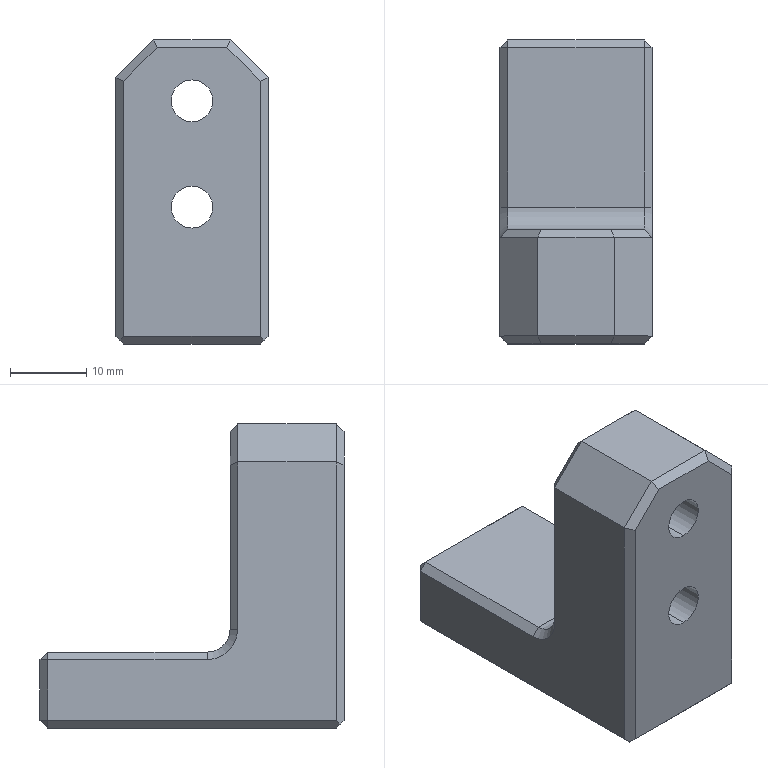Part | Creo | 1 solid | 46 faces | box 20 x 40 x 40 mm | volume 15202 mm3 | plane 35 | cylinder 9 | cone 2 | commonest cylinder face diameters 5.5 x4 9.5 x4 6 x1
STEP:
#1=CARTESIAN_POINT('',(-227.177,374.995,-9.5));
#2=VERTEX_POINT('',#1);
#3=CARTESIAN_POINT('',(-227.177,374.995,24.086));
#4=VERTEX_POINT('',#3);
#5=CARTESIAN_POINT('',(-227.177,374.995,-9.5));
#6=DIRECTION('',(0.,0.,1.));
#7=VECTOR('',#6,33.586);
#8=LINE('',#5,#7);
#9=EDGE_CURVE('',#2,#4,#8,.T.);
#10=ORIENTED_EDGE('',*,*,#9,.T.);
#11=CARTESIAN_POINT('',(-222.763,374.995,28.5));
#12=VERTEX_POINT('',#11);
#13=CARTESIAN_POINT('',(-222.763,374.995,28.5));
#14=DIRECTION('',(-0.7071,0.,-0.7071));
#15=VECTOR('',#14,6.243);
#16=LINE('',#13,#15);
#17=EDGE_CURVE('',#12,#4,#16,.T.);
#18=ORIENTED_EDGE('',*,*,#17,.F.);
#19=CARTESIAN_POINT('',(-213.591,374.995,28.5));
#20=VERTEX_POINT('',#19);
#21=CARTESIAN_POINT('',(-222.763,374.995,28.5));
#22=DIRECTION('',(1.,0.,0.));
#23=VECTOR('',#22,9.172);
#24=LINE('',#21,#23);
#25=EDGE_CURVE('',#12,#20,#24,.T.);
#26=ORIENTED_EDGE('',*,*,#25,.T.);
#27=CARTESIAN_POINT('',(-209.177,374.995,24.086));
#28=VERTEX_POINT('',#27);
#29=CARTESIAN_POINT('',(-209.177,374.995,24.086));
#30=DIRECTION('',(-0.7071,0.,0.7071));
#31=VECTOR('',#30,6.243);
#32=LINE('',#29,#31);
#33=EDGE_CURVE('',#28,#20,#32,.T.);
#34=ORIENTED_EDGE('',*,*,#33,.F.);
#35=CARTESIAN_POINT('',(-209.177,374.995,-9.5));
#36=VERTEX_POINT('',#35);
#37=CARTESIAN_POINT('',(-209.177,374.995,24.086));
#38=DIRECTION('',(0.,0.,-1.));
#39=VECTOR('',#38,33.586);
#40=LINE('',#37,#39);
#41=EDGE_CURVE('',#28,#36,#40,.T.);
#42=ORIENTED_EDGE('',*,*,#41,.T.);
#43=CARTESIAN_POINT('',(-209.177,374.995,-9.5));
#44=DIRECTION('',(-1.,0.,0.));
#45=VECTOR('',#44,18.);
#46=LINE('',#43,#45);
#47=EDGE_CURVE('',#36,#2,#46,.T.);
#48=ORIENTED_EDGE('',*,*,#47,.T.);
#49=EDGE_LOOP('',(#10,#18,#26,#34,#42,#48));
#50=FACE_OUTER_BOUND('',#49,.F.);
#51=CARTESIAN_POINT('',(-218.177,374.995,4.75));
#52=VERTEX_POINT('',#51);
#53=CARTESIAN_POINT('',(-218.177,374.995,10.25));
#54=VERTEX_POINT('',#53);
#55=CARTESIAN_POINT('',(-218.177,374.995,7.5));
#56=DIRECTION('',(0.,1.,0.));
#57=DIRECTION('',(0.,0.,-1.));
#58=AXIS2_PLACEMENT_3D('',#55,#56,#57);
#59=CIRCLE('',#58,2.75);
#60=EDGE_CURVE('',#52,#54,#59,.T.);
#61=ORIENTED_EDGE('',*,*,#60,.F.);
#62=CARTESIAN_POINT('',(-218.177,374.995,7.5));
#63=DIRECTION('',(0.,1.,0.));
#64=DIRECTION('',(0.,0.,1.));
#65=AXIS2_PLACEMENT_3D('',#62,#63,#64);
#66=CIRCLE('',#65,2.75);
#67=EDGE_CURVE('',#54,#52,#66,.T.);
#68=ORIENTED_EDGE('',*,*,#67,.F.);
#69=EDGE_LOOP('',(#61,#68));
#70=FACE_BOUND('',#69,.F.);
#71=CARTESIAN_POINT('',(-218.177,374.995,18.75));
#72=VERTEX_POINT('',#71);
#73=CARTESIAN_POINT('',(-218.177,374.995,24.25));
#74=VERTEX_POINT('',#73);
#75=CARTESIAN_POINT('',(-218.177,374.995,21.5));
#76=DIRECTION('',(0.,1.,0.));
#77=DIRECTION('',(0.,0.,-1.));
#78=AXIS2_PLACEMENT_3D('',#75,#76,#77);
#79=CIRCLE('',#78,2.75);
#80=EDGE_CURVE('',#72,#74,#79,.T.);
#81=ORIENTED_EDGE('',*,*,#80,.F.);
#82=CARTESIAN_POINT('',(-218.177,374.995,21.5));
#83=DIRECTION('',(0.,1.,0.));
#84=DIRECTION('',(0.,0.,1.));
#85=AXIS2_PLACEMENT_3D('',#82,#83,#84);
#86=CIRCLE('',#85,2.75);
#87=EDGE_CURVE('',#74,#72,#86,.T.);
#88=ORIENTED_EDGE('',*,*,#87,.F.);
#89=EDGE_LOOP('',(#81,#88));
#90=FACE_BOUND('',#89,.F.);
#91=CARTESIAN_POINT('',(-218.177,374.995,12.));
#92=DIRECTION('',(0.,-1.,0.));
#93=DIRECTION('',(0.,0.,-1.));
#94=AXIS2_PLACEMENT_3D('',#91,#92,#93);
#95=PLANE('',#94);
#96=ADVANCED_FACE('',(#50,#70,#90),#95,.T.);
#97=ORIENTED_EDGE('',*,*,#60,.T.);
#98=CARTESIAN_POINT('',(-218.177,383.995,10.25));
#99=VERTEX_POINT('',#98);
#100=CARTESIAN_POINT('',(-218.177,374.995,10.25));
#101=DIRECTION('',(0.,1.,0.));
#102=VECTOR('',#101,9.);
#103=LINE('',#100,#102);
#104=EDGE_CURVE('',#54,#99,#103,.T.);
#105=ORIENTED_EDGE('',*,*,#104,.T.);
#106=CARTESIAN_POINT('',(-218.177,383.995,4.75));
#107=VERTEX_POINT('',#106);
#108=CARTESIAN_POINT('',(-218.177,383.995,7.5));
#109=DIRECTION('',(0.,-1.,0.));
#110=DIRECTION('',(0.,0.,1.));
#111=AXIS2_PLACEMENT_3D('',#108,#109,#110);
#112=CIRCLE('',#111,2.75);
#113=EDGE_CURVE('',#99,#107,#112,.T.);
#114=ORIENTED_EDGE('',*,*,#113,.T.);
#115=CARTESIAN_POINT('',(-218.177,374.995,4.75));
#116=DIRECTION('',(0.,1.,0.));
#117=VECTOR('',#116,9.);
#118=LINE('',#115,#117);
#119=EDGE_CURVE('',#52,#107,#118,.T.);
#120=ORIENTED_EDGE('',*,*,#119,.F.);
#121=EDGE_LOOP('',(#97,#105,#114,#120));
#122=FACE_OUTER_BOUND('',#121,.F.);
#123=CARTESIAN_POINT('',(-218.177,389.995,7.5));
#124=DIRECTION('',(0.,1.,0.));
#125=DIRECTION('',(0.,0.,1.));
#126=AXIS2_PLACEMENT_3D('',#123,#124,#125);
#127=CYLINDRICAL_SURFACE('',#126,2.75);
#128=ADVANCED_FACE('',(#122),#127,.F.);
#129=ORIENTED_EDGE('',*,*,#67,.T.);
#130=ORIENTED_EDGE('',*,*,#119,.T.);
#131=CARTESIAN_POINT('',(-218.177,383.995,7.5));
#132=DIRECTION('',(0.,-1.,0.));
#133=DIRECTION('',(0.,0.,-1.));
#134=AXIS2_PLACEMENT_3D('',#131,#132,#133);
#135=CIRCLE('',#134,2.75);
#136=EDGE_CURVE('',#107,#99,#135,.T.);
#137=ORIENTED_EDGE('',*,*,#136,.T.);
#138=ORIENTED_EDGE('',*,*,#104,.F.);
#139=EDGE_LOOP('',(#129,#130,#137,#138));
#140=FACE_OUTER_BOUND('',#139,.F.);
#141=CARTESIAN_POINT('',(-218.177,389.995,7.5));
#142=DIRECTION('',(0.,1.,0.));
#143=DIRECTION('',(0.,0.,1.));
#144=AXIS2_PLACEMENT_3D('',#141,#142,#143);
#145=CYLINDRICAL_SURFACE('',#144,2.75);
#146=ADVANCED_FACE('',(#140),#145,.F.);
#147=CARTESIAN_POINT('',(-218.177,383.995,2.75));
#148=VERTEX_POINT('',#147);
#149=CARTESIAN_POINT('',(-218.177,383.995,12.25));
#150=VERTEX_POINT('',#149);
#151=CARTESIAN_POINT('',(-218.177,383.995,7.5));
#152=DIRECTION('',(0.,1.,0.));
#153=DIRECTION('',(0.,0.,-1.));
#154=AXIS2_PLACEMENT_3D('',#151,#152,#153);
#155=CIRCLE('',#154,4.75);
#156=EDGE_CURVE('',#148,#150,#155,.T.);
#157=ORIENTED_EDGE('',*,*,#156,.F.);
#158=CARTESIAN_POINT('',(-218.177,383.995,7.5));
#159=DIRECTION('',(0.,1.,0.));
#160=DIRECTION('',(0.,0.,1.));
#161=AXIS2_PLACEMENT_3D('',#158,#159,#160);
#162=CIRCLE('',#161,4.75);
#163=EDGE_CURVE('',#150,#148,#162,.T.);
#164=ORIENTED_EDGE('',*,*,#163,.F.);
#165=EDGE_LOOP('',(#157,#164));
#166=FACE_OUTER_BOUND('',#165,.F.);
#167=ORIENTED_EDGE('',*,*,#136,.F.);
#168=ORIENTED_EDGE('',*,*,#113,.F.);
#169=EDGE_LOOP('',(#167,#168));
#170=FACE_BOUND('',#169,.F.);
#171=CARTESIAN_POINT('',(-222.927,383.995,7.5));
#172=DIRECTION('',(0.,-1.,0.));
#173=DIRECTION('',(0.,0.,-1.));
#174=AXIS2_PLACEMENT_3D('',#171,#172,#173);
#175=PLANE('',#174);
#176=ADVANCED_FACE('',(#166,#170),#175,.F.);
#177=ORIENTED_EDGE('',*,*,#156,.T.);
#178=CARTESIAN_POINT('',(-218.177,389.995,12.25));
#179=VERTEX_POINT('',#178);
#180=CARTESIAN_POINT('',(-218.177,383.995,12.25));
#181=DIRECTION('',(0.,1.,0.));
#182=VECTOR('',#181,6.);
#183=LINE('',#180,#182);
#184=EDGE_CURVE('',#150,#179,#183,.T.);
#185=ORIENTED_EDGE('',*,*,#184,.T.);
#186=CARTESIAN_POINT('',(-218.177,389.995,2.75));
#187=VERTEX_POINT('',#186);
#188=CARTESIAN_POINT('',(-218.177,389.995,7.5));
#189=DIRECTION('',(0.,-1.,0.));
#190=DIRECTION('',(0.,0.,1.));
#191=AXIS2_PLACEMENT_3D('',#188,#189,#190);
#192=CIRCLE('',#191,4.75);
#193=EDGE_CURVE('',#179,#187,#192,.T.);
#194=ORIENTED_EDGE('',*,*,#193,.T.);
#195=CARTESIAN_POINT('',(-218.177,383.995,2.75));
#196=DIRECTION('',(0.,1.,0.));
#197=VECTOR('',#196,6.);
#198=LINE('',#195,#197);
#199=EDGE_CURVE('',#148,#187,#198,.T.);
#200=ORIENTED_EDGE('',*,*,#199,.F.);
#201=EDGE_LOOP('',(#177,#185,#194,#200));
#202=FACE_OUTER_BOUND('',#201,.F.);
#203=CARTESIAN_POINT('',(-218.177,389.995,7.5));
#204=DIRECTION('',(0.,1.,0.));
#205=DIRECTION('',(0.,0.,1.));
#206=AXIS2_PLACEMENT_3D('',#203,#204,#205);
#207=CYLINDRICAL_SURFACE('',#206,4.75);
#208=ADVANCED_FACE('',(#202),#207,.F.);
#209=ORIENTED_EDGE('',*,*,#163,.T.);
#210=ORIENTED_EDGE('',*,*,#199,.T.);
#211=CARTESIAN_POINT('',(-218.177,389.995,7.5));
#212=DIRECTION('',(0.,-1.,0.));
#213=DIRECTION('',(0.,0.,-1.));
#214=AXIS2_PLACEMENT_3D('',#211,#212,#213);
#215=CIRCLE('',#214,4.75);
#216=EDGE_CURVE('',#187,#179,#215,.T.);
#217=ORIENTED_EDGE('',*,*,#216,.T.);
#218=ORIENTED_EDGE('',*,*,#184,.F.);
#219=EDGE_LOOP('',(#209,#210,#217,#218));
#220=FACE_OUTER_BOUND('',#219,.F.);
#221=CARTESIAN_POINT('',(-218.177,389.995,7.5));
#222=DIRECTION('',(0.,1.,0.));
#223=DIRECTION('',(0.,0.,1.));
#224=AXIS2_PLACEMENT_3D('',#221,#222,#223);
#225=CYLINDRICAL_SURFACE('',#224,4.75);
#226=ADVANCED_FACE('',(#220),#225,.F.);
#227=CARTESIAN_POINT('',(-213.591,389.995,28.5));
#228=VERTEX_POINT('',#227);
#229=CARTESIAN_POINT('',(-209.177,389.995,24.086));
#230=VERTEX_POINT('',#229);
#231=CARTESIAN_POINT('',(-213.591,389.995,28.5));
#232=DIRECTION('',(0.7071,0.,-0.7071));
#233=VECTOR('',#232,6.243);
#234=LINE('',#231,#233);
#235=EDGE_CURVE('',#228,#230,#234,.T.);
#236=ORIENTED_EDGE('',*,*,#235,.F.);
#237=CARTESIAN_POINT('',(-222.763,389.995,28.5));
#238=VERTEX_POINT('',#237);
#239=CARTESIAN_POINT('',(-213.591,389.995,28.5));
#240=DIRECTION('',(-1.,0.,0.));
#241=VECTOR('',#240,9.172);
#242=LINE('',#239,#241);
#243=EDGE_CURVE('',#228,#238,#242,.T.);
#244=ORIENTED_EDGE('',*,*,#243,.T.);
#245=CARTESIAN_POINT('',(-227.177,389.995,24.086));
#246=VERTEX_POINT('',#245);
#247=CARTESIAN_POINT('',(-227.177,389.995,24.086));
#248=DIRECTION('',(0.7071,0.,0.7071));
#249=VECTOR('',#248,6.243);
#250=LINE('',#247,#249);
#251=EDGE_CURVE('',#246,#238,#250,.T.);
#252=ORIENTED_EDGE('',*,*,#251,.F.);
#253=CARTESIAN_POINT('',(-227.177,389.995,2.5));
#254=VERTEX_POINT('',#253);
#255=CARTESIAN_POINT('',(-227.177,389.995,24.086));
#256=DIRECTION('',(0.,0.,-1.));
#257=VECTOR('',#256,21.586);
#258=LINE('',#255,#257);
#259=EDGE_CURVE('',#246,#254,#258,.T.);
#260=ORIENTED_EDGE('',*,*,#259,.T.);
#261=CARTESIAN_POINT('',(-209.177,389.995,2.5));
#262=VERTEX_POINT('',#261);
#263=CARTESIAN_POINT('',(-227.177,389.995,2.5));
#264=DIRECTION('',(1.,0.,0.));
#265=VECTOR('',#264,18.);
#266=LINE('',#263,#265);
#267=EDGE_CURVE('',#254,#262,#266,.T.);
#268=ORIENTED_EDGE('',*,*,#267,.T.);
#269=CARTESIAN_POINT('',(-209.177,389.995,2.5));
#270=DIRECTION('',(0.,0.,1.));
#271=VECTOR('',#270,21.586);
#272=LINE('',#269,#271);
#273=EDGE_CURVE('',#262,#230,#272,.T.);
#274=ORIENTED_EDGE('',*,*,#273,.T.);
#275=EDGE_LOOP('',(#236,#244,#252,#260,#268,#274));
#276=FACE_OUTER_BOUND('',#275,.F.);
#277=ORIENTED_EDGE('',*,*,#216,.F.);
#278=ORIENTED_EDGE('',*,*,#193,.F.);
#279=EDGE_LOOP('',(#277,#278));
#280=FACE_BOUND('',#279,.F.);
#281=CARTESIAN_POINT('',(-218.177,389.995,16.75));
#282=VERTEX_POINT('',#281);
#283=CARTESIAN_POINT('',(-218.177,389.995,26.25));
#284=VERTEX_POINT('',#283);
#285=CARTESIAN_POINT('',(-218.177,389.995,21.5));
#286=DIRECTION('',(0.,-1.,0.));
#287=DIRECTION('',(0.,0.,-1.));
#288=AXIS2_PLACEMENT_3D('',#285,#286,#287);
#289=CIRCLE('',#288,4.75);
#290=EDGE_CURVE('',#282,#284,#289,.T.);
#291=ORIENTED_EDGE('',*,*,#290,.F.);
#292=CARTESIAN_POINT('',(-218.177,389.995,21.5));
#293=DIRECTION('',(0.,-1.,0.));
#294=DIRECTION('',(0.,0.,1.));
#295=AXIS2_PLACEMENT_3D('',#292,#293,#294);
#296=CIRCLE('',#295,4.75);
#297=EDGE_CURVE('',#284,#282,#296,.T.);
#298=ORIENTED_EDGE('',*,*,#297,.F.);
#299=EDGE_LOOP('',(#291,#298));
#300=FACE_BOUND('',#299,.F.);
#301=CARTESIAN_POINT('',(-218.177,389.995,27.));
#302=DIRECTION('',(0.,-1.,0.));
#303=DIRECTION('',(0.,0.,-1.));
#304=AXIS2_PLACEMENT_3D('',#301,#302,#303);
#305=PLANE('',#304);
#306=ADVANCED_FACE('',(#276,#280,#300),#305,.F.);
#307=CARTESIAN_POINT('',(-213.177,388.995,29.5));
#308=VERTEX_POINT('',#307);
#309=CARTESIAN_POINT('',(-213.177,388.995,29.5));
#310=DIRECTION('',(-0.2811,0.6786,-0.6786));
#311=VECTOR('',#310,1.474);
#312=LINE('',#309,#311);
#313=EDGE_CURVE('',#308,#228,#312,.T.);
#314=ORIENTED_EDGE('',*,*,#313,.T.);
#315=ORIENTED_EDGE('',*,*,#235,.T.);
#316=CARTESIAN_POINT('',(-208.177,388.995,24.5));
#317=VERTEX_POINT('',#316);
#318=CARTESIAN_POINT('',(-208.177,388.995,24.5));
#319=DIRECTION('',(-0.6786,0.6786,-0.2811));
#320=VECTOR('',#319,1.474);
#321=LINE('',#318,#320);
#322=EDGE_CURVE('',#317,#230,#321,.T.);
#323=ORIENTED_EDGE('',*,*,#322,.F.);
#324=CARTESIAN_POINT('',(-213.177,388.995,29.5));
#325=DIRECTION('',(0.7071,0.,-0.7071));
#326=VECTOR('',#325,7.071);
#327=LINE('',#324,#326);
#328=EDGE_CURVE('',#308,#317,#327,.T.);
#329=ORIENTED_EDGE('',*,*,#328,.F.);
#330=EDGE_LOOP('',(#314,#315,#323,#329));
#331=FACE_OUTER_BOUND('',#330,.F.);
#332=CARTESIAN_POINT('',(-212.634,389.995,27.543));
#333=DIRECTION('',(-0.5,-0.7071,-0.5));
#334=DIRECTION('',(-0.7071,0.,0.7071));
#335=AXIS2_PLACEMENT_3D('',#332,#333,#334);
#336=PLANE('',#335);
#337=ADVANCED_FACE('',(#331),#336,.F.);
#338=ORIENTED_EDGE('',*,*,#313,.F.);
#339=CARTESIAN_POINT('',(-223.177,388.995,29.5));
#340=VERTEX_POINT('',#339);
#341=CARTESIAN_POINT('',(-223.177,388.995,29.5));
#342=DIRECTION('',(1.,0.,0.));
#343=VECTOR('',#342,10.);
#344=LINE('',#341,#343);
#345=EDGE_CURVE('',#340,#308,#344,.T.);
#346=ORIENTED_EDGE('',*,*,#345,.F.);
#347=CARTESIAN_POINT('',(-222.763,389.995,28.5));
#348=DIRECTION('',(-0.2811,-0.6786,0.6786));
#349=VECTOR('',#348,1.474);
#350=LINE('',#347,#349);
#351=EDGE_CURVE('',#238,#340,#350,.T.);
#352=ORIENTED_EDGE('',*,*,#351,.F.);
#353=ORIENTED_EDGE('',*,*,#243,.F.);
#354=EDGE_LOOP('',(#338,#346,#352,#353));
#355=FACE_OUTER_BOUND('',#354,.F.);
#356=CARTESIAN_POINT('',(-218.177,389.995,28.5));
#357=DIRECTION('',(0.,0.7071,0.7071));
#358=DIRECTION('',(1.,0.,0.));
#359=AXIS2_PLACEMENT_3D('',#356,#357,#358);
#360=PLANE('',#359);
#361=ADVANCED_FACE('',(#355),#360,.T.);
#362=CARTESIAN_POINT('',(-213.177,375.995,29.5));
#363=VERTEX_POINT('',#362);
#364=CARTESIAN_POINT('',(-213.177,388.995,29.5));
#365=DIRECTION('',(0.,-1.,0.));
#366=VECTOR('',#365,13.);
#367=LINE('',#364,#366);
#368=EDGE_CURVE('',#308,#363,#367,.T.);
#369=ORIENTED_EDGE('',*,*,#368,.T.);
#370=CARTESIAN_POINT('',(-223.177,375.995,29.5));
#371=VERTEX_POINT('',#370);
#372=CARTESIAN_POINT('',(-213.177,375.995,29.5));
#373=DIRECTION('',(-1.,0.,0.));
#374=VECTOR('',#373,10.);
#375=LINE('',#372,#374);
#376=EDGE_CURVE('',#363,#371,#375,.T.);
#377=ORIENTED_EDGE('',*,*,#376,.T.);
#378=CARTESIAN_POINT('',(-223.177,375.995,29.5));
#379=DIRECTION('',(0.,1.,0.));
#380=VECTOR('',#379,13.);
#381=LINE('',#378,#380);
#382=EDGE_CURVE('',#371,#340,#381,.T.);
#383=ORIENTED_EDGE('',*,*,#382,.T.);
#384=ORIENTED_EDGE('',*,*,#345,.T.);
#385=EDGE_LOOP('',(#369,#377,#383,#384));
#386=FACE_OUTER_BOUND('',#385,.F.);
#387=CARTESIAN_POINT('',(-218.177,333.995,29.5));
#388=DIRECTION('',(0.,0.,1.));
#389=DIRECTION('',(0.,-1.,0.));
#390=AXIS2_PLACEMENT_3D('',#387,#388,#389);
#391=PLANE('',#390);
#392=ADVANCED_FACE('',(#386),#391,.T.);
#393=ORIENTED_EDGE('',*,*,#368,.F.);
#394=ORIENTED_EDGE('',*,*,#328,.T.);
#395=CARTESIAN_POINT('',(-208.177,375.995,24.5));
#396=VERTEX_POINT('',#395);
#397=CARTESIAN_POINT('',(-208.177,375.995,24.5));
#398=DIRECTION('',(0.,1.,0.));
#399=VECTOR('',#398,13.);
#400=LINE('',#397,#399);
#401=EDGE_CURVE('',#396,#317,#400,.T.);
#402=ORIENTED_EDGE('',*,*,#401,.F.);
#403=CARTESIAN_POINT('',(-208.177,375.995,24.5));
#404=DIRECTION('',(-0.7071,0.,0.7071));
#405=VECTOR('',#404,7.071);
#406=LINE('',#403,#405);
#407=EDGE_CURVE('',#396,#363,#406,.T.);
#408=ORIENTED_EDGE('',*,*,#407,.T.);
#409=EDGE_LOOP('',(#393,#394,#402,#408));
#410=FACE_OUTER_BOUND('',#409,.F.);
#411=CARTESIAN_POINT('',(-213.177,333.995,29.5));
#412=DIRECTION('',(-0.7071,0.,-0.7071));
#413=DIRECTION('',(0.,-1.,0.));
#414=AXIS2_PLACEMENT_3D('',#411,#412,#413);
#415=PLANE('',#414);
#416=ADVANCED_FACE('',(#410),#415,.F.);
#417=ORIENTED_EDGE('',*,*,#401,.T.);
#418=CARTESIAN_POINT('',(-208.177,388.995,2.5));
#419=VERTEX_POINT('',#418);
#420=CARTESIAN_POINT('',(-208.177,388.995,24.5));
#421=DIRECTION('',(0.,0.,-1.));
#422=VECTOR('',#421,22.);
#423=LINE('',#420,#422);
#424=EDGE_CURVE('',#317,#419,#423,.T.);
#425=ORIENTED_EDGE('',*,*,#424,.T.);
#426=CARTESIAN_POINT('',(-208.177,392.995,-1.5));
#427=VERTEX_POINT('',#426);
#428=CARTESIAN_POINT('',(-208.177,392.995,2.5));
#429=DIRECTION('',(-1.,0.,0.));
#430=DIRECTION('',(0.,0.,-1.));
#431=AXIS2_PLACEMENT_3D('',#428,#429,#430);
#432=CIRCLE('',#431,4.);
#433=EDGE_CURVE('',#427,#419,#432,.T.);
#434=ORIENTED_EDGE('',*,*,#433,.F.);
#435=CARTESIAN_POINT('',(-208.177,413.995,-1.5));
#436=VERTEX_POINT('',#435);
#437=CARTESIAN_POINT('',(-208.177,392.995,-1.5));
#438=DIRECTION('',(0.,1.,0.));
#439=VECTOR('',#438,21.);
#440=LINE('',#437,#439);
#441=EDGE_CURVE('',#427,#436,#440,.T.);
#442=ORIENTED_EDGE('',*,*,#441,.T.);
#443=CARTESIAN_POINT('',(-208.177,413.995,-9.5));
#444=VERTEX_POINT('',#443);
#445=CARTESIAN_POINT('',(-208.177,413.995,-1.5));
#446=DIRECTION('',(0.,0.,-1.));
#447=VECTOR('',#446,8.);
#448=LINE('',#445,#447);
#449=EDGE_CURVE('',#436,#444,#448,.T.);
#450=ORIENTED_EDGE('',*,*,#449,.T.);
#451=CARTESIAN_POINT('',(-208.177,375.995,-9.5));
#452=VERTEX_POINT('',#451);
#453=CARTESIAN_POINT('',(-208.177,413.995,-9.5));
#454=DIRECTION('',(0.,-1.,0.));
#455=VECTOR('',#454,38.);
#456=LINE('',#453,#455);
#457=EDGE_CURVE('',#444,#452,#456,.T.);
#458=ORIENTED_EDGE('',*,*,#457,.T.);
#459=CARTESIAN_POINT('',(-208.177,375.995,-9.5));
#460=DIRECTION('',(0.,0.,1.));
#461=VECTOR('',#460,34.);
#462=LINE('',#459,#461);
#463=EDGE_CURVE('',#452,#396,#462,.T.);
#464=ORIENTED_EDGE('',*,*,#463,.T.);
#465=EDGE_LOOP('',(#417,#425,#434,#442,#450,#458,#464));
#466=FACE_OUTER_BOUND('',#465,.F.);
#467=CARTESIAN_POINT('',(-208.177,333.995,12.));
#468=DIRECTION('',(1.,0.,0.));
#469=DIRECTION('',(0.,1.,0.));
#470=AXIS2_PLACEMENT_3D('',#467,#468,#469);
#471=PLANE('',#470);
#472=ADVANCED_FACE('',(#466),#471,.T.);
#473=ORIENTED_EDGE('',*,*,#322,.T.);
#474=ORIENTED_EDGE('',*,*,#273,.F.);
#475=CARTESIAN_POINT('',(-209.177,389.995,2.5));
#476=DIRECTION('',(0.7071,-0.7071,0.));
#477=VECTOR('',#476,1.414);
#478=LINE('',#475,#477);
#479=EDGE_CURVE('',#262,#419,#478,.T.);
#480=ORIENTED_EDGE('',*,*,#479,.T.);
#481=ORIENTED_EDGE('',*,*,#424,.F.);
#482=EDGE_LOOP('',(#473,#474,#480,#481));
#483=FACE_OUTER_BOUND('',#482,.F.);
#484=CARTESIAN_POINT('',(-209.177,389.995,27.));
#485=DIRECTION('',(0.7071,0.7071,0.));
#486=DIRECTION('',(0.,0.,-1.));
#487=AXIS2_PLACEMENT_3D('',#484,#485,#486);
#488=PLANE('',#487);
#489=ADVANCED_FACE('',(#483),#488,.T.);
#490=ORIENTED_EDGE('',*,*,#479,.F.);
#491=CARTESIAN_POINT('',(-209.177,392.995,-0.5));
#492=VERTEX_POINT('',#491);
#493=CARTESIAN_POINT('',(-209.177,392.995,2.5));
#494=DIRECTION('',(-1.,0.,0.));
#495=DIRECTION('',(0.,0.,-1.));
#496=AXIS2_PLACEMENT_3D('',#493,#494,#495);
#497=CIRCLE('',#496,3.);
#498=EDGE_CURVE('',#492,#262,#497,.T.);
#499=ORIENTED_EDGE('',*,*,#498,.F.);
#500=CARTESIAN_POINT('',(-208.177,392.995,-1.5));
#501=DIRECTION('',(-0.7071,0.,0.7071));
#502=VECTOR('',#501,1.414);
#503=LINE('',#500,#502);
#504=EDGE_CURVE('',#427,#492,#503,.T.);
#505=ORIENTED_EDGE('',*,*,#504,.F.);
#506=ORIENTED_EDGE('',*,*,#433,.T.);
#507=EDGE_LOOP('',(#490,#499,#505,#506));
#508=FACE_OUTER_BOUND('',#507,.F.);
#509=CARTESIAN_POINT('',(-208.677,392.995,2.5));
#510=DIRECTION('',(1.,0.,0.));
#511=DIRECTION('',(0.,1.,0.));
#512=AXIS2_PLACEMENT_3D('',#509,#510,#511);
#513=CONICAL_SURFACE('',#512,3.5,45.);
#514=ADVANCED_FACE('',(#508),#513,.F.);
#515=ORIENTED_EDGE('',*,*,#267,.F.);
#516=CARTESIAN_POINT('',(-227.177,392.995,-0.5));
#517=VERTEX_POINT('',#516);
#518=CARTESIAN_POINT('',(-227.177,392.995,2.5));
#519=DIRECTION('',(1.,0.,0.));
#520=DIRECTION('',(0.,-1.,0.));
#521=AXIS2_PLACEMENT_3D('',#518,#519,#520);
#522=CIRCLE('',#521,3.);
#523=EDGE_CURVE('',#254,#517,#522,.T.);
#524=ORIENTED_EDGE('',*,*,#523,.T.);
#525=CARTESIAN_POINT('',(-209.177,392.995,-0.5));
#526=DIRECTION('',(-1.,0.,0.));
#527=VECTOR('',#526,18.);
#528=LINE('',#525,#527);
#529=EDGE_CURVE('',#492,#517,#528,.T.);
#530=ORIENTED_EDGE('',*,*,#529,.F.);
#531=ORIENTED_EDGE('',*,*,#498,.T.);
#532=EDGE_LOOP('',(#515,#524,#530,#531));
#533=FACE_OUTER_BOUND('',#532,.F.);
#534=CARTESIAN_POINT('',(-218.177,392.995,2.5));
#535=DIRECTION('',(-1.,0.,0.));
#536=DIRECTION('',(0.,-1.,0.));
#537=AXIS2_PLACEMENT_3D('',#534,#535,#536);
#538=CYLINDRICAL_SURFACE('',#537,3.);
#539=ADVANCED_FACE('',(#533),#538,.F.);
#540=CARTESIAN_POINT('',(-228.177,388.995,2.5));
#541=VERTEX_POINT('',#540);
#542=CARTESIAN_POINT('',(-228.177,388.995,2.5));
#543=DIRECTION('',(0.7071,0.7071,0.));
#544=VECTOR('',#543,1.414);
#545=LINE('',#542,#544);
#546=EDGE_CURVE('',#541,#254,#545,.T.);
#547=ORIENTED_EDGE('',*,*,#546,.F.);
#548=CARTESIAN_POINT('',(-228.177,392.995,-1.5));
#549=VERTEX_POINT('',#548);
#550=CARTESIAN_POINT('',(-228.177,392.995,2.5));
#551=DIRECTION('',(1.,0.,0.));
#552=DIRECTION('',(0.,-1.,0.));
#553=AXIS2_PLACEMENT_3D('',#550,#551,#552);
#554=CIRCLE('',#553,4.);
#555=EDGE_CURVE('',#541,#549,#554,.T.);
#556=ORIENTED_EDGE('',*,*,#555,.T.);
#557=CARTESIAN_POINT('',(-227.177,392.995,-0.5));
#558=DIRECTION('',(-0.7071,0.,-0.7071));
#559=VECTOR('',#558,1.414);
#560=LINE('',#557,#559);
#561=EDGE_CURVE('',#517,#549,#560,.T.);
#562=ORIENTED_EDGE('',*,*,#561,.F.);
#563=ORIENTED_EDGE('',*,*,#523,.F.);
#564=EDGE_LOOP('',(#547,#556,#562,#563));
#565=FACE_OUTER_BOUND('',#564,.F.);
#566=CARTESIAN_POINT('',(-227.677,392.995,2.5));
#567=DIRECTION('',(-1.,0.,0.));
#568=DIRECTION('',(0.,-1.,0.));
#569=AXIS2_PLACEMENT_3D('',#566,#567,#568);
#570=CONICAL_SURFACE('',#569,3.5,45.);
#571=ADVANCED_FACE('',(#565),#570,.F.);
#572=CARTESIAN_POINT('',(-228.177,388.995,24.5));
#573=VERTEX_POINT('',#572);
#574=CARTESIAN_POINT('',(-227.177,389.995,24.086));
#575=DIRECTION('',(-0.6786,-0.6786,0.2811));
#576=VECTOR('',#575,1.474);
#577=LINE('',#574,#576);
#578=EDGE_CURVE('',#246,#573,#577,.T.);
#579=ORIENTED_EDGE('',*,*,#578,.T.);
#580=CARTESIAN_POINT('',(-228.177,388.995,2.5));
#581=DIRECTION('',(0.,0.,1.));
#582=VECTOR('',#581,22.);
#583=LINE('',#580,#582);
#584=EDGE_CURVE('',#541,#573,#583,.T.);
#585=ORIENTED_EDGE('',*,*,#584,.F.);
#586=ORIENTED_EDGE('',*,*,#546,.T.);
#587=ORIENTED_EDGE('',*,*,#259,.F.);
#588=EDGE_LOOP('',(#579,#585,#586,#587));
#589=FACE_OUTER_BOUND('',#588,.F.);
#590=CARTESIAN_POINT('',(-227.177,389.995,27.));
#591=DIRECTION('',(-0.7071,0.7071,0.));
#592=DIRECTION('',(0.,0.,1.));
#593=AXIS2_PLACEMENT_3D('',#590,#591,#592);
#594=PLANE('',#593);
#595=ADVANCED_FACE('',(#589),#594,.T.);
#596=ORIENTED_EDGE('',*,*,#351,.T.);
#597=CARTESIAN_POINT('',(-228.177,388.995,24.5));
#598=DIRECTION('',(0.7071,0.,0.7071));
#599=VECTOR('',#598,7.071);
#600=LINE('',#597,#599);
#601=EDGE_CURVE('',#573,#340,#600,.T.);
#602=ORIENTED_EDGE('',*,*,#601,.F.);
#603=ORIENTED_EDGE('',*,*,#578,.F.);
#604=ORIENTED_EDGE('',*,*,#251,.T.);
#605=EDGE_LOOP('',(#596,#602,#603,#604));
#606=FACE_OUTER_BOUND('',#605,.F.);
#607=CARTESIAN_POINT('',(-223.72,389.995,27.543));
#608=DIRECTION('',(0.5,-0.7071,-0.5));
#609=DIRECTION('',(-0.7071,0.,-0.7071));
#610=AXIS2_PLACEMENT_3D('',#607,#608,#609);
#611=PLANE('',#610);
#612=ADVANCED_FACE('',(#606),#611,.F.);
#613=ORIENTED_EDGE('',*,*,#382,.F.);
#614=CARTESIAN_POINT('',(-228.177,375.995,24.5));
#615=VERTEX_POINT('',#614);
#616=CARTESIAN_POINT('',(-223.177,375.995,29.5));
#617=DIRECTION('',(-0.7071,0.,-0.7071));
#618=VECTOR('',#617,7.071);
#619=LINE('',#616,#618);
#620=EDGE_CURVE('',#371,#615,#619,.T.);
#621=ORIENTED_EDGE('',*,*,#620,.T.);
#622=CARTESIAN_POINT('',(-228.177,388.995,24.5));
#623=DIRECTION('',(0.,-1.,0.));
#624=VECTOR('',#623,13.);
#625=LINE('',#622,#624);
#626=EDGE_CURVE('',#573,#615,#625,.T.);
#627=ORIENTED_EDGE('',*,*,#626,.F.);
#628=ORIENTED_EDGE('',*,*,#601,.T.);
#629=EDGE_LOOP('',(#613,#621,#627,#628));
#630=FACE_OUTER_BOUND('',#629,.F.);
#631=CARTESIAN_POINT('',(-228.177,333.995,24.5));
#632=DIRECTION('',(0.7071,0.,-0.7071));
#633=DIRECTION('',(0.,-1.,0.));
#634=AXIS2_PLACEMENT_3D('',#631,#632,#633);
#635=PLANE('',#634);
#636=ADVANCED_FACE('',(#630),#635,.F.);
#637=CARTESIAN_POINT('',(-223.177,375.995,29.5));
#638=DIRECTION('',(0.2811,-0.6786,-0.6786));
#639=VECTOR('',#638,1.474);
#640=LINE('',#637,#639);
#641=EDGE_CURVE('',#371,#12,#640,.T.);
#642=ORIENTED_EDGE('',*,*,#641,.T.);
#643=ORIENTED_EDGE('',*,*,#17,.T.);
#644=CARTESIAN_POINT('',(-228.177,375.995,24.5));
#645=DIRECTION('',(0.6786,-0.6786,-0.2811));
#646=VECTOR('',#645,1.474);
#647=LINE('',#644,#646);
#648=EDGE_CURVE('',#615,#4,#647,.T.);
#649=ORIENTED_EDGE('',*,*,#648,.F.);
#650=ORIENTED_EDGE('',*,*,#620,.F.);
#651=EDGE_LOOP('',(#642,#643,#649,#650));
#652=FACE_OUTER_BOUND('',#651,.F.);
#653=CARTESIAN_POINT('',(-231.22,374.995,20.043));
#654=DIRECTION('',(-0.5,-0.7071,0.5));
#655=DIRECTION('',(-0.7071,0.,-0.7071));
#656=AXIS2_PLACEMENT_3D('',#653,#654,#655);
#657=PLANE('',#656);
#658=ADVANCED_FACE('',(#652),#657,.T.);
#659=CARTESIAN_POINT('',(-213.591,374.995,28.5));
#660=DIRECTION('',(0.2811,0.6786,0.6786));
#661=VECTOR('',#660,1.474);
#662=LINE('',#659,#661);
#663=EDGE_CURVE('',#20,#363,#662,.T.);
#664=ORIENTED_EDGE('',*,*,#663,.F.);
#665=ORIENTED_EDGE('',*,*,#25,.F.);
#666=ORIENTED_EDGE('',*,*,#641,.F.);
#667=ORIENTED_EDGE('',*,*,#376,.F.);
#668=EDGE_LOOP('',(#664,#665,#666,#667));
#669=FACE_OUTER_BOUND('',#668,.F.);
#670=CARTESIAN_POINT('',(-218.177,375.995,29.5));
#671=DIRECTION('',(0.,0.7071,-0.7071));
#672=DIRECTION('',(-1.,0.,0.));
#673=AXIS2_PLACEMENT_3D('',#670,#671,#672);
#674=PLANE('',#673);
#675=ADVANCED_FACE('',(#669),#674,.F.);
#676=ORIENTED_EDGE('',*,*,#663,.T.);
#677=ORIENTED_EDGE('',*,*,#407,.F.);
#678=CARTESIAN_POINT('',(-209.177,374.995,24.086));
#679=DIRECTION('',(0.6786,0.6786,0.2811));
#680=VECTOR('',#679,1.474);
#681=LINE('',#678,#680);
#682=EDGE_CURVE('',#28,#396,#681,.T.);
#683=ORIENTED_EDGE('',*,*,#682,.F.);
#684=ORIENTED_EDGE('',*,*,#33,.T.);
#685=EDGE_LOOP('',(#676,#677,#683,#684));
#686=FACE_OUTER_BOUND('',#685,.F.);
#687=CARTESIAN_POINT('',(-205.134,374.995,20.043));
#688=DIRECTION('',(0.5,-0.7071,0.5));
#689=DIRECTION('',(-0.7071,0.,0.7071));
#690=AXIS2_PLACEMENT_3D('',#687,#688,#689);
#691=PLANE('',#690);
#692=ADVANCED_FACE('',(#686),#691,.T.);
#693=ORIENTED_EDGE('',*,*,#41,.F.);
#694=ORIENTED_EDGE('',*,*,#682,.T.);
#695=ORIENTED_EDGE('',*,*,#463,.F.);
#696=CARTESIAN_POINT('',(-208.677,375.495,-10.));
#697=VERTEX_POINT('',#696);
#698=CARTESIAN_POINT('',(-208.677,375.495,-10.));
#699=DIRECTION('',(0.5774,0.5774,0.5774));
#700=VECTOR('',#699,0.866);
#701=LINE('',#698,#700);
#702=EDGE_CURVE('',#697,#452,#701,.T.);
#703=ORIENTED_EDGE('',*,*,#702,.F.);
#704=CARTESIAN_POINT('',(-208.677,375.495,-10.));
#705=DIRECTION('',(-0.5774,-0.5774,0.5774));
#706=VECTOR('',#705,0.866);
#707=LINE('',#704,#706);
#708=EDGE_CURVE('',#697,#36,#707,.T.);
#709=ORIENTED_EDGE('',*,*,#708,.T.);
#710=EDGE_LOOP('',(#693,#694,#695,#703,#709));
#711=FACE_OUTER_BOUND('',#710,.F.);
#712=CARTESIAN_POINT('',(-208.177,375.995,12.));
#713=DIRECTION('',(-0.7071,0.7071,0.));
#714=DIRECTION('',(0.,0.,1.));
#715=AXIS2_PLACEMENT_3D('',#712,#713,#714);
#716=PLANE('',#715);
#717=ADVANCED_FACE('',(#711),#716,.F.);
#718=ORIENTED_EDGE('',*,*,#702,.T.);
#719=ORIENTED_EDGE('',*,*,#457,.F.);
#720=CARTESIAN_POINT('',(-209.177,413.995,-10.5));
#721=VERTEX_POINT('',#720);
#722=CARTESIAN_POINT('',(-208.177,413.995,-9.5));
#723=DIRECTION('',(-0.7071,0.,-0.7071));
#724=VECTOR('',#723,1.414);
#725=LINE('',#722,#724);
#726=EDGE_CURVE('',#444,#721,#725,.T.);
#727=ORIENTED_EDGE('',*,*,#726,.T.);
#728=CARTESIAN_POINT('',(-209.177,375.995,-10.5));
#729=VERTEX_POINT('',#728);
#730=CARTESIAN_POINT('',(-209.177,375.995,-10.5));
#731=DIRECTION('',(0.,1.,0.));
#732=VECTOR('',#731,38.);
#733=LINE('',#730,#732);
#734=EDGE_CURVE('',#729,#721,#733,.T.);
#735=ORIENTED_EDGE('',*,*,#734,.F.);
#736=CARTESIAN_POINT('',(-209.177,375.995,-10.5));
#737=DIRECTION('',(0.5774,-0.5774,0.5774));
#738=VECTOR('',#737,0.866);
#739=LINE('',#736,#738);
#740=EDGE_CURVE('',#729,#697,#739,.T.);
#741=ORIENTED_EDGE('',*,*,#740,.T.);
#742=EDGE_LOOP('',(#718,#719,#727,#735,#741));
#743=FACE_OUTER_BOUND('',#742,.F.);
#744=CARTESIAN_POINT('',(-208.177,333.995,-9.5));
#745=DIRECTION('',(-0.7071,0.,0.7071));
#746=DIRECTION('',(0.,-1.,0.));
#747=AXIS2_PLACEMENT_3D('',#744,#745,#746);
#748=PLANE('',#747);
#749=ADVANCED_FACE('',(#743),#748,.F.);
#750=CARTESIAN_POINT('',(-209.177,414.995,-9.5));
#751=VERTEX_POINT('',#750);
#752=CARTESIAN_POINT('',(-209.177,414.995,-9.5));
#753=DIRECTION('',(0.7071,-0.7071,0.));
#754=VECTOR('',#753,1.414);
#755=LINE('',#752,#754);
#756=EDGE_CURVE('',#751,#444,#755,.T.);
#757=ORIENTED_EDGE('',*,*,#756,.F.);
#758=CARTESIAN_POINT('',(-209.177,413.995,-10.5));
#759=DIRECTION('',(0.,0.7071,0.7071));
#760=VECTOR('',#759,1.414);
#761=LINE('',#758,#760);
#762=EDGE_CURVE('',#721,#751,#761,.T.);
#763=ORIENTED_EDGE('',*,*,#762,.F.);
#764=ORIENTED_EDGE('',*,*,#726,.F.);
#765=EDGE_LOOP('',(#757,#763,#764));
#766=FACE_OUTER_BOUND('',#765,.F.);
#767=CARTESIAN_POINT('',(-209.177,413.995,-10.5));
#768=DIRECTION('',(0.5774,0.5774,-0.5774));
#769=DIRECTION('',(0.,0.7071,0.7071));
#770=AXIS2_PLACEMENT_3D('',#767,#768,#769);
#771=PLANE('',#770);
#772=ADVANCED_FACE('',(#766),#771,.T.);
#773=CARTESIAN_POINT('',(-209.177,414.995,-1.5));
#774=VERTEX_POINT('',#773);
#775=CARTESIAN_POINT('',(-208.177,413.995,-1.5));
#776=DIRECTION('',(-0.7071,0.7071,0.));
#777=VECTOR('',#776,1.414);
#778=LINE('',#775,#777);
#779=EDGE_CURVE('',#436,#774,#778,.T.);
#780=ORIENTED_EDGE('',*,*,#779,.T.);
#781=CARTESIAN_POINT('',(-209.177,414.995,-9.5));
#782=DIRECTION('',(0.,0.,1.));
#783=VECTOR('',#782,8.);
#784=LINE('',#781,#783);
#785=EDGE_CURVE('',#751,#774,#784,.T.);
#786=ORIENTED_EDGE('',*,*,#785,.F.);
#787=ORIENTED_EDGE('',*,*,#756,.T.);
#788=ORIENTED_EDGE('',*,*,#449,.F.);
#789=EDGE_LOOP('',(#780,#786,#787,#788));
#790=FACE_OUTER_BOUND('',#789,.F.);
#791=CARTESIAN_POINT('',(-208.177,413.995,12.));
#792=DIRECTION('',(-0.7071,-0.7071,0.));
#793=DIRECTION('',(0.,0.,-1.));
#794=AXIS2_PLACEMENT_3D('',#791,#792,#793);
#795=PLANE('',#794);
#796=ADVANCED_FACE('',(#790),#795,.F.);
#797=CARTESIAN_POINT('',(-209.177,413.995,-0.5));
#798=VERTEX_POINT('',#797);
#799=CARTESIAN_POINT('',(-209.177,413.995,-0.5));
#800=DIRECTION('',(0.,0.7071,-0.7071));
#801=VECTOR('',#800,1.414);
#802=LINE('',#799,#801);
#803=EDGE_CURVE('',#798,#774,#802,.T.);
#804=ORIENTED_EDGE('',*,*,#803,.T.);
#805=ORIENTED_EDGE('',*,*,#779,.F.);
#806=CARTESIAN_POINT('',(-209.177,413.995,-0.5));
#807=DIRECTION('',(0.7071,0.,-0.7071));
#808=VECTOR('',#807,1.414);
#809=LINE('',#806,#808);
#810=EDGE_CURVE('',#798,#436,#809,.T.);
#811=ORIENTED_EDGE('',*,*,#810,.F.);
#812=EDGE_LOOP('',(#804,#805,#811));
#813=FACE_OUTER_BOUND('',#812,.F.);
#814=CARTESIAN_POINT('',(-208.177,413.995,-1.5));
#815=DIRECTION('',(0.5774,0.5774,0.5774));
#816=DIRECTION('',(0.,-0.7071,0.7071));
#817=AXIS2_PLACEMENT_3D('',#814,#815,#816);
#818=PLANE('',#817);
#819=ADVANCED_FACE('',(#813),#818,.T.);
#820=CARTESIAN_POINT('',(-227.177,414.995,-1.5));
#821=VERTEX_POINT('',#820);
#822=CARTESIAN_POINT('',(-227.177,413.995,-0.5));
#823=VERTEX_POINT('',#822);
#824=CARTESIAN_POINT('',(-227.177,414.995,-1.5));
#825=DIRECTION('',(0.,-0.7071,0.7071));
#826=VECTOR('',#825,1.414);
#827=LINE('',#824,#826);
#828=EDGE_CURVE('',#821,#823,#827,.T.);
#829=ORIENTED_EDGE('',*,*,#828,.F.);
#830=CARTESIAN_POINT('',(-209.177,414.995,-1.5));
#831=DIRECTION('',(-1.,0.,0.));
#832=VECTOR('',#831,18.);
#833=LINE('',#830,#832);
#834=EDGE_CURVE('',#774,#821,#833,.T.);
#835=ORIENTED_EDGE('',*,*,#834,.F.);
#836=ORIENTED_EDGE('',*,*,#803,.F.);
#837=CARTESIAN_POINT('',(-227.177,413.995,-0.5));
#838=DIRECTION('',(1.,0.,0.));
#839=VECTOR('',#838,18.);
#840=LINE('',#837,#839);
#841=EDGE_CURVE('',#823,#798,#840,.T.);
#842=ORIENTED_EDGE('',*,*,#841,.F.);
#843=EDGE_LOOP('',(#829,#835,#836,#842));
#844=FACE_OUTER_BOUND('',#843,.F.);
#845=CARTESIAN_POINT('',(-218.177,413.995,-0.5));
#846=DIRECTION('',(0.,0.7071,0.7071));
#847=DIRECTION('',(-1.,0.,0.));
#848=AXIS2_PLACEMENT_3D('',#845,#846,#847);
#849=PLANE('',#848);
#850=ADVANCED_FACE('',(#844),#849,.T.);
#851=CARTESIAN_POINT('',(-228.177,413.995,-1.5));
#852=VERTEX_POINT('',#851);
#853=CARTESIAN_POINT('',(-228.177,413.995,-1.5));
#854=DIRECTION('',(0.7071,0.,0.7071));
#855=VECTOR('',#854,1.414);
#856=LINE('',#853,#855);
#857=EDGE_CURVE('',#852,#823,#856,.T.);
#858=ORIENTED_EDGE('',*,*,#857,.F.);
#859=CARTESIAN_POINT('',(-227.177,414.995,-1.5));
#860=DIRECTION('',(-0.7071,-0.7071,0.));
#861=VECTOR('',#860,1.414);
#862=LINE('',#859,#861);
#863=EDGE_CURVE('',#821,#852,#862,.T.);
#864=ORIENTED_EDGE('',*,*,#863,.F.);
#865=ORIENTED_EDGE('',*,*,#828,.T.);
#866=EDGE_LOOP('',(#858,#864,#865));
#867=FACE_OUTER_BOUND('',#866,.F.);
#868=CARTESIAN_POINT('',(-228.177,413.995,-1.5));
#869=DIRECTION('',(-0.5774,0.5774,0.5774));
#870=DIRECTION('',(0.,-0.7071,0.7071));
#871=AXIS2_PLACEMENT_3D('',#868,#869,#870);
#872=PLANE('',#871);
#873=ADVANCED_FACE('',(#867),#872,.T.);
#874=ORIENTED_EDGE('',*,*,#561,.T.);
#875=CARTESIAN_POINT('',(-228.177,413.995,-1.5));
#876=DIRECTION('',(0.,-1.,0.));
#877=VECTOR('',#876,21.);
#878=LINE('',#875,#877);
#879=EDGE_CURVE('',#852,#549,#878,.T.);
#880=ORIENTED_EDGE('',*,*,#879,.F.);
#881=ORIENTED_EDGE('',*,*,#857,.T.);
#882=CARTESIAN_POINT('',(-227.177,392.995,-0.5));
#883=DIRECTION('',(0.,1.,0.));
#884=VECTOR('',#883,21.);
#885=LINE('',#882,#884);
#886=EDGE_CURVE('',#517,#823,#885,.T.);
#887=ORIENTED_EDGE('',*,*,#886,.F.);
#888=EDGE_LOOP('',(#874,#880,#881,#887));
#889=FACE_OUTER_BOUND('',#888,.F.);
#890=CARTESIAN_POINT('',(-227.177,389.995,-0.5));
#891=DIRECTION('',(-0.7071,0.,0.7071));
#892=DIRECTION('',(0.,-1.,0.));
#893=AXIS2_PLACEMENT_3D('',#890,#891,#892);
#894=PLANE('',#893);
#895=ADVANCED_FACE('',(#889),#894,.T.);
#896=ORIENTED_EDGE('',*,*,#626,.T.);
#897=CARTESIAN_POINT('',(-228.177,375.995,-9.5));
#898=VERTEX_POINT('',#897);
#899=CARTESIAN_POINT('',(-228.177,375.995,24.5));
#900=DIRECTION('',(0.,0.,-1.));
#901=VECTOR('',#900,34.);
#902=LINE('',#899,#901);
#903=EDGE_CURVE('',#615,#898,#902,.T.);
#904=ORIENTED_EDGE('',*,*,#903,.T.);
#905=CARTESIAN_POINT('',(-228.177,413.995,-9.5));
#906=VERTEX_POINT('',#905);
#907=CARTESIAN_POINT('',(-228.177,375.995,-9.5));
#908=DIRECTION('',(0.,1.,0.));
#909=VECTOR('',#908,38.);
#910=LINE('',#907,#909);
#911=EDGE_CURVE('',#898,#906,#910,.T.);
#912=ORIENTED_EDGE('',*,*,#911,.T.);
#913=CARTESIAN_POINT('',(-228.177,413.995,-9.5));
#914=DIRECTION('',(0.,0.,1.));
#915=VECTOR('',#914,8.);
#916=LINE('',#913,#915);
#917=EDGE_CURVE('',#906,#852,#916,.T.);
#918=ORIENTED_EDGE('',*,*,#917,.T.);
#919=ORIENTED_EDGE('',*,*,#879,.T.);
#920=ORIENTED_EDGE('',*,*,#555,.F.);
#921=ORIENTED_EDGE('',*,*,#584,.T.);
#922=EDGE_LOOP('',(#896,#904,#912,#918,#919,#920,#921));
#923=FACE_OUTER_BOUND('',#922,.F.);
#924=CARTESIAN_POINT('',(-228.177,333.995,12.));
#925=DIRECTION('',(-1.,0.,0.));
#926=DIRECTION('',(0.,-1.,0.));
#927=AXIS2_PLACEMENT_3D('',#924,#925,#926);
#928=PLANE('',#927);
#929=ADVANCED_FACE('',(#923),#928,.T.);
#930=CARTESIAN_POINT('',(-227.677,375.495,-10.));
#931=VERTEX_POINT('',#930);
#932=CARTESIAN_POINT('',(-228.177,375.995,-9.5));
#933=DIRECTION('',(0.5774,-0.5774,-0.5774));
#934=VECTOR('',#933,0.866);
#935=LINE('',#932,#934);
#936=EDGE_CURVE('',#898,#931,#935,.T.);
#937=ORIENTED_EDGE('',*,*,#936,.F.);
#938=ORIENTED_EDGE('',*,*,#903,.F.);
#939=ORIENTED_EDGE('',*,*,#648,.T.);
#940=ORIENTED_EDGE('',*,*,#9,.F.);
#941=CARTESIAN_POINT('',(-227.177,374.995,-9.5));
#942=DIRECTION('',(-0.5774,0.5774,-0.5774));
#943=VECTOR('',#942,0.866);
#944=LINE('',#941,#943);
#945=EDGE_CURVE('',#2,#931,#944,.T.);
#946=ORIENTED_EDGE('',*,*,#945,.T.);
#947=EDGE_LOOP('',(#937,#938,#939,#940,#946));
#948=FACE_OUTER_BOUND('',#947,.F.);
#949=CARTESIAN_POINT('',(-228.177,375.995,12.));
#950=DIRECTION('',(0.7071,0.7071,0.));
#951=DIRECTION('',(0.,0.,-1.));
#952=AXIS2_PLACEMENT_3D('',#949,#950,#951);
#953=PLANE('',#952);
#954=ADVANCED_FACE('',(#948),#953,.F.);
#955=CARTESIAN_POINT('',(-227.177,413.995,-10.5));
#956=VERTEX_POINT('',#955);
#957=CARTESIAN_POINT('',(-227.177,375.995,-10.5));
#958=VERTEX_POINT('',#957);
#959=CARTESIAN_POINT('',(-227.177,413.995,-10.5));
#960=DIRECTION('',(0.,-1.,0.));
#961=VECTOR('',#960,38.);
#962=LINE('',#959,#961);
#963=EDGE_CURVE('',#956,#958,#962,.T.);
#964=ORIENTED_EDGE('',*,*,#963,.F.);
#965=CARTESIAN_POINT('',(-227.177,413.995,-10.5));
#966=DIRECTION('',(-0.7071,0.,0.7071));
#967=VECTOR('',#966,1.414);
#968=LINE('',#965,#967);
#969=EDGE_CURVE('',#956,#906,#968,.T.);
#970=ORIENTED_EDGE('',*,*,#969,.T.);
#971=ORIENTED_EDGE('',*,*,#911,.F.);
#972=ORIENTED_EDGE('',*,*,#936,.T.);
#973=CARTESIAN_POINT('',(-227.677,375.495,-10.));
#974=DIRECTION('',(0.5774,0.5774,-0.5774));
#975=VECTOR('',#974,0.866);
#976=LINE('',#973,#975);
#977=EDGE_CURVE('',#931,#958,#976,.T.);
#978=ORIENTED_EDGE('',*,*,#977,.T.);
#979=EDGE_LOOP('',(#964,#970,#971,#972,#978));
#980=FACE_OUTER_BOUND('',#979,.F.);
#981=CARTESIAN_POINT('',(-227.177,333.995,-10.5));
#982=DIRECTION('',(0.7071,0.,0.7071));
#983=DIRECTION('',(0.,-1.,0.));
#984=AXIS2_PLACEMENT_3D('',#981,#982,#983);
#985=PLANE('',#984);
#986=ADVANCED_FACE('',(#980),#985,.F.);
#987=ORIENTED_EDGE('',*,*,#734,.T.);
#988=CARTESIAN_POINT('',(-209.177,413.995,-10.5));
#989=DIRECTION('',(-1.,0.,0.));
#990=VECTOR('',#989,18.);
#991=LINE('',#988,#990);
#992=EDGE_CURVE('',#721,#956,#991,.T.);
#993=ORIENTED_EDGE('',*,*,#992,.T.);
#994=ORIENTED_EDGE('',*,*,#963,.T.);
#995=CARTESIAN_POINT('',(-227.177,375.995,-10.5));
#996=DIRECTION('',(1.,0.,0.));
#997=VECTOR('',#996,18.);
#998=LINE('',#995,#997);
#999=EDGE_CURVE('',#958,#729,#998,.T.);
#1000=ORIENTED_EDGE('',*,*,#999,.T.);
#1001=EDGE_LOOP('',(#987,#993,#994,#1000));
#1002=FACE_OUTER_BOUND('',#1001,.F.);
#1003=CARTESIAN_POINT('',(-218.177,333.995,-10.5));
#1004=DIRECTION('',(0.,0.,-1.));
#1005=DIRECTION('',(0.,1.,0.));
#1006=AXIS2_PLACEMENT_3D('',#1003,#1004,#1005);
#1007=PLANE('',#1006);
#1008=ADVANCED_FACE('',(#1002),#1007,.T.);
#1009=CARTESIAN_POINT('',(-227.177,414.995,-9.5));
#1010=VERTEX_POINT('',#1009);
#1011=CARTESIAN_POINT('',(-227.177,414.995,-9.5));
#1012=DIRECTION('',(0.,-0.7071,-0.7071));
#1013=VECTOR('',#1012,1.414);
#1014=LINE('',#1011,#1013);
#1015=EDGE_CURVE('',#1010,#956,#1014,.T.);
#1016=ORIENTED_EDGE('',*,*,#1015,.T.);
#1017=ORIENTED_EDGE('',*,*,#992,.F.);
#1018=ORIENTED_EDGE('',*,*,#762,.T.);
#1019=CARTESIAN_POINT('',(-227.177,414.995,-9.5));
#1020=DIRECTION('',(1.,0.,0.));
#1021=VECTOR('',#1020,18.);
#1022=LINE('',#1019,#1021);
#1023=EDGE_CURVE('',#1010,#751,#1022,.T.);
#1024=ORIENTED_EDGE('',*,*,#1023,.F.);
#1025=EDGE_LOOP('',(#1016,#1017,#1018,#1024));
#1026=FACE_OUTER_BOUND('',#1025,.F.);
#1027=CARTESIAN_POINT('',(-218.177,413.995,-10.5));
#1028=DIRECTION('',(0.,-0.7071,0.7071));
#1029=DIRECTION('',(-1.,0.,0.));
#1030=AXIS2_PLACEMENT_3D('',#1027,#1028,#1029);
#1031=PLANE('',#1030);
#1032=ADVANCED_FACE('',(#1026),#1031,.F.);
#1033=ORIENTED_EDGE('',*,*,#969,.F.);
#1034=ORIENTED_EDGE('',*,*,#1015,.F.);
#1035=CARTESIAN_POINT('',(-228.177,413.995,-9.5));
#1036=DIRECTION('',(0.7071,0.7071,0.));
#1037=VECTOR('',#1036,1.414);
#1038=LINE('',#1035,#1037);
#1039=EDGE_CURVE('',#906,#1010,#1038,.T.);
#1040=ORIENTED_EDGE('',*,*,#1039,.F.);
#1041=EDGE_LOOP('',(#1033,#1034,#1040));
#1042=FACE_OUTER_BOUND('',#1041,.F.);
#1043=CARTESIAN_POINT('',(-227.177,414.995,-9.5));
#1044=DIRECTION('',(-0.5774,0.5774,-0.5774));
#1045=DIRECTION('',(0.,0.7071,0.7071));
#1046=AXIS2_PLACEMENT_3D('',#1043,#1044,#1045);
#1047=PLANE('',#1046);
#1048=ADVANCED_FACE('',(#1042),#1047,.T.);
#1049=ORIENTED_EDGE('',*,*,#863,.T.);
#1050=ORIENTED_EDGE('',*,*,#917,.F.);
#1051=ORIENTED_EDGE('',*,*,#1039,.T.);
#1052=CARTESIAN_POINT('',(-227.177,414.995,-1.5));
#1053=DIRECTION('',(0.,0.,-1.));
#1054=VECTOR('',#1053,8.);
#1055=LINE('',#1052,#1054);
#1056=EDGE_CURVE('',#821,#1010,#1055,.T.);
#1057=ORIENTED_EDGE('',*,*,#1056,.F.);
#1058=EDGE_LOOP('',(#1049,#1050,#1051,#1057));
#1059=FACE_OUTER_BOUND('',#1058,.F.);
#1060=CARTESIAN_POINT('',(-228.177,413.995,12.));
#1061=DIRECTION('',(0.7071,-0.7071,0.));
#1062=DIRECTION('',(0.,0.,1.));
#1063=AXIS2_PLACEMENT_3D('',#1060,#1061,#1062);
#1064=PLANE('',#1063);
#1065=ADVANCED_FACE('',(#1059),#1064,.F.);
#1066=ORIENTED_EDGE('',*,*,#785,.T.);
#1067=ORIENTED_EDGE('',*,*,#834,.T.);
#1068=ORIENTED_EDGE('',*,*,#1056,.T.);
#1069=ORIENTED_EDGE('',*,*,#1023,.T.);
#1070=EDGE_LOOP('',(#1066,#1067,#1068,#1069));
#1071=FACE_OUTER_BOUND('',#1070,.F.);
#1072=CARTESIAN_POINT('',(-218.177,414.995,12.));
#1073=DIRECTION('',(0.,1.,0.));
#1074=DIRECTION('',(0.,0.,1.));
#1075=AXIS2_PLACEMENT_3D('',#1072,#1073,#1074);
#1076=PLANE('',#1075);
#1077=ADVANCED_FACE('',(#1071),#1076,.T.);
#1078=ORIENTED_EDGE('',*,*,#708,.F.);
#1079=ORIENTED_EDGE('',*,*,#740,.F.);
#1080=ORIENTED_EDGE('',*,*,#999,.F.);
#1081=ORIENTED_EDGE('',*,*,#977,.F.);
#1082=ORIENTED_EDGE('',*,*,#945,.F.);
#1083=ORIENTED_EDGE('',*,*,#47,.F.);
#1084=EDGE_LOOP('',(#1078,#1079,#1080,#1081,#1082,#1083));
#1085=FACE_OUTER_BOUND('',#1084,.F.);
#1086=CARTESIAN_POINT('',(-218.177,375.995,-10.5));
#1087=DIRECTION('',(0.,0.7071,0.7071));
#1088=DIRECTION('',(1.,0.,0.));
#1089=AXIS2_PLACEMENT_3D('',#1086,#1087,#1088);
#1090=PLANE('',#1089);
#1091=ADVANCED_FACE('',(#1085),#1090,.F.);
#1092=ORIENTED_EDGE('',*,*,#529,.T.);
#1093=ORIENTED_EDGE('',*,*,#886,.T.);
#1094=ORIENTED_EDGE('',*,*,#841,.T.);
#1095=CARTESIAN_POINT('',(-209.177,413.995,-0.5));
#1096=DIRECTION('',(0.,-1.,0.));
#1097=VECTOR('',#1096,21.);
#1098=LINE('',#1095,#1097);
#1099=EDGE_CURVE('',#798,#492,#1098,.T.);
#1100=ORIENTED_EDGE('',*,*,#1099,.T.);
#1101=EDGE_LOOP('',(#1092,#1093,#1094,#1100));
#1102=FACE_OUTER_BOUND('',#1101,.F.);
#1103=CARTESIAN_POINT('',(-218.177,389.995,-0.5));
#1104=DIRECTION('',(0.,0.,-1.));
#1105=DIRECTION('',(0.,1.,0.));
#1106=AXIS2_PLACEMENT_3D('',#1103,#1104,#1105);
#1107=PLANE('',#1106);
#1108=ADVANCED_FACE('',(#1102),#1107,.F.);
#1109=ORIENTED_EDGE('',*,*,#504,.T.);
#1110=ORIENTED_EDGE('',*,*,#1099,.F.);
#1111=ORIENTED_EDGE('',*,*,#810,.T.);
#1112=ORIENTED_EDGE('',*,*,#441,.F.);
#1113=EDGE_LOOP('',(#1109,#1110,#1111,#1112));
#1114=FACE_OUTER_BOUND('',#1113,.F.);
#1115=CARTESIAN_POINT('',(-209.177,389.995,-0.5));
#1116=DIRECTION('',(0.7071,0.,0.7071));
#1117=DIRECTION('',(0.,1.,0.));
#1118=AXIS2_PLACEMENT_3D('',#1115,#1116,#1117);
#1119=PLANE('',#1118);
#1120=ADVANCED_FACE('',(#1114),#1119,.T.);
#1121=CARTESIAN_POINT('',(-218.177,383.995,26.25));
#1122=VERTEX_POINT('',#1121);
#1123=CARTESIAN_POINT('',(-218.177,383.995,16.75));
#1124=VERTEX_POINT('',#1123);
#1125=CARTESIAN_POINT('',(-218.177,383.995,21.5));
#1126=DIRECTION('',(0.,1.,0.));
#1127=DIRECTION('',(0.,0.,1.));
#1128=AXIS2_PLACEMENT_3D('',#1125,#1126,#1127);
#1129=CIRCLE('',#1128,4.75);
#1130=EDGE_CURVE('',#1122,#1124,#1129,.T.);
#1131=ORIENTED_EDGE('',*,*,#1130,.T.);
#1132=CARTESIAN_POINT('',(-218.177,383.995,16.75));
#1133=DIRECTION('',(0.,1.,0.));
#1134=VECTOR('',#1133,6.);
#1135=LINE('',#1132,#1134);
#1136=EDGE_CURVE('',#1124,#282,#1135,.T.);
#1137=ORIENTED_EDGE('',*,*,#1136,.T.);
#1138=ORIENTED_EDGE('',*,*,#290,.T.);
#1139=CARTESIAN_POINT('',(-218.177,383.995,26.25));
#1140=DIRECTION('',(0.,1.,0.));
#1141=VECTOR('',#1140,6.);
#1142=LINE('',#1139,#1141);
#1143=EDGE_CURVE('',#1122,#284,#1142,.T.);
#1144=ORIENTED_EDGE('',*,*,#1143,.F.);
#1145=EDGE_LOOP('',(#1131,#1137,#1138,#1144));
#1146=FACE_OUTER_BOUND('',#1145,.F.);
#1147=CARTESIAN_POINT('',(-218.177,389.995,21.5));
#1148=DIRECTION('',(0.,1.,0.));
#1149=DIRECTION('',(0.,0.,1.));
#1150=AXIS2_PLACEMENT_3D('',#1147,#1148,#1149);
#1151=CYLINDRICAL_SURFACE('',#1150,4.75);
#1152=ADVANCED_FACE('',(#1146),#1151,.F.);
#1153=CARTESIAN_POINT('',(-218.177,383.995,21.5));
#1154=DIRECTION('',(0.,1.,0.));
#1155=DIRECTION('',(0.,0.,-1.));
#1156=AXIS2_PLACEMENT_3D('',#1153,#1154,#1155);
#1157=CIRCLE('',#1156,4.75);
#1158=EDGE_CURVE('',#1124,#1122,#1157,.T.);
#1159=ORIENTED_EDGE('',*,*,#1158,.F.);
#1160=ORIENTED_EDGE('',*,*,#1130,.F.);
#1161=EDGE_LOOP('',(#1159,#1160));
#1162=FACE_OUTER_BOUND('',#1161,.F.);
#1163=CARTESIAN_POINT('',(-218.177,383.995,18.75));
#1164=VERTEX_POINT('',#1163);
#1165=CARTESIAN_POINT('',(-218.177,383.995,24.25));
#1166=VERTEX_POINT('',#1165);
#1167=CARTESIAN_POINT('',(-218.177,383.995,21.5));
#1168=DIRECTION('',(0.,-1.,0.));
#1169=DIRECTION('',(0.,0.,-1.));
#1170=AXIS2_PLACEMENT_3D('',#1167,#1168,#1169);
#1171=CIRCLE('',#1170,2.75);
#1172=EDGE_CURVE('',#1164,#1166,#1171,.T.);
#1173=ORIENTED_EDGE('',*,*,#1172,.F.);
#1174=CARTESIAN_POINT('',(-218.177,383.995,21.5));
#1175=DIRECTION('',(0.,-1.,0.));
#1176=DIRECTION('',(0.,0.,1.));
#1177=AXIS2_PLACEMENT_3D('',#1174,#1175,#1176);
#1178=CIRCLE('',#1177,2.75);
#1179=EDGE_CURVE('',#1166,#1164,#1178,.T.);
#1180=ORIENTED_EDGE('',*,*,#1179,.F.);
#1181=EDGE_LOOP('',(#1173,#1180));
#1182=FACE_BOUND('',#1181,.F.);
#1183=CARTESIAN_POINT('',(-222.927,383.995,21.5));
#1184=DIRECTION('',(0.,-1.,0.));
#1185=DIRECTION('',(0.,0.,-1.));
#1186=AXIS2_PLACEMENT_3D('',#1183,#1184,#1185);
#1187=PLANE('',#1186);
#1188=ADVANCED_FACE('',(#1162,#1182),#1187,.F.);
#1189=ORIENTED_EDGE('',*,*,#87,.T.);
#1190=CARTESIAN_POINT('',(-218.177,374.995,18.75));
#1191=DIRECTION('',(0.,1.,0.));
#1192=VECTOR('',#1191,9.);
#1193=LINE('',#1190,#1192);
#1194=EDGE_CURVE('',#72,#1164,#1193,.T.);
#1195=ORIENTED_EDGE('',*,*,#1194,.T.);
#1196=ORIENTED_EDGE('',*,*,#1172,.T.);
#1197=CARTESIAN_POINT('',(-218.177,374.995,24.25));
#1198=DIRECTION('',(0.,1.,0.));
#1199=VECTOR('',#1198,9.);
#1200=LINE('',#1197,#1199);
#1201=EDGE_CURVE('',#74,#1166,#1200,.T.);
#1202=ORIENTED_EDGE('',*,*,#1201,.F.);
#1203=EDGE_LOOP('',(#1189,#1195,#1196,#1202));
#1204=FACE_OUTER_BOUND('',#1203,.F.);
#1205=CARTESIAN_POINT('',(-218.177,389.995,21.5));
#1206=DIRECTION('',(0.,1.,0.));
#1207=DIRECTION('',(0.,0.,1.));
#1208=AXIS2_PLACEMENT_3D('',#1205,#1206,#1207);
#1209=CYLINDRICAL_SURFACE('',#1208,2.75);
#1210=ADVANCED_FACE('',(#1204),#1209,.F.);
#1211=ORIENTED_EDGE('',*,*,#80,.T.);
#1212=ORIENTED_EDGE('',*,*,#1201,.T.);
#1213=ORIENTED_EDGE('',*,*,#1179,.T.);
#1214=ORIENTED_EDGE('',*,*,#1194,.F.);
#1215=EDGE_LOOP('',(#1211,#1212,#1213,#1214));
#1216=FACE_OUTER_BOUND('',#1215,.F.);
#1217=CARTESIAN_POINT('',(-218.177,389.995,21.5));
#1218=DIRECTION('',(0.,1.,0.));
#1219=DIRECTION('',(0.,0.,1.));
#1220=AXIS2_PLACEMENT_3D('',#1217,#1218,#1219);
#1221=CYLINDRICAL_SURFACE('',#1220,2.75);
#1222=ADVANCED_FACE('',(#1216),#1221,.F.);
#1223=ORIENTED_EDGE('',*,*,#1158,.T.);
#1224=ORIENTED_EDGE('',*,*,#1143,.T.);
#1225=ORIENTED_EDGE('',*,*,#297,.T.);
#1226=ORIENTED_EDGE('',*,*,#1136,.F.);
#1227=EDGE_LOOP('',(#1223,#1224,#1225,#1226));
#1228=FACE_OUTER_BOUND('',#1227,.F.);
#1229=CARTESIAN_POINT('',(-218.177,389.995,21.5));
#1230=DIRECTION('',(0.,1.,0.));
#1231=DIRECTION('',(0.,0.,1.));
#1232=AXIS2_PLACEMENT_3D('',#1229,#1230,#1231);
#1233=CYLINDRICAL_SURFACE('',#1232,4.75);
#1234=ADVANCED_FACE('',(#1228),#1233,.F.);
#1235=CLOSED_SHELL('',(#96,#128,#146,#176,#208,#226,#306,#337,#361,#392,#416,#472,#489,#514,#539,#571,#595,#612,#636,#658,#675,#692,#717,#749,#772,#796,#819,#850,#873,#895,#929,#954,#986,#1008,#1032,#1048,#1065,#1077,#1091,#1108,#1120,#1152,#1188,#1210,#1222,#1234));
#1236=MANIFOLD_SOLID_BREP('',#1235);
#1237=(LENGTH_UNIT()NAMED_UNIT(*)SI_UNIT(.MILLI.,.METRE.));
#1238=UNCERTAINTY_MEASURE_WITH_UNIT(LENGTH_MEASURE(0.006),#1237,'','');
#1239=(NAMED_UNIT(*)PLANE_ANGLE_UNIT()SI_UNIT($,.RADIAN.));
#1240=PLANE_ANGLE_MEASURE_WITH_UNIT(PLANE_ANGLE_MEASURE(0.01745),#1239);
#1241=(CONVERSION_BASED_UNIT('DEGREE',#1240)NAMED_UNIT(*)PLANE_ANGLE_UNIT());
#1242=(NAMED_UNIT(*)SI_UNIT($,.STERADIAN.)SOLID_ANGLE_UNIT());
#1243=(GEOMETRIC_REPRESENTATION_CONTEXT(3)GLOBAL_UNCERTAINTY_ASSIGNED_CONTEXT((#1238))GLOBAL_UNIT_ASSIGNED_CONTEXT((#1237,#1241,#1242))REPRESENTATION_CONTEXT('',''));
#1244=ADVANCED_BREP_SHAPE_REPRESENTATION('',(#1236),#1243);